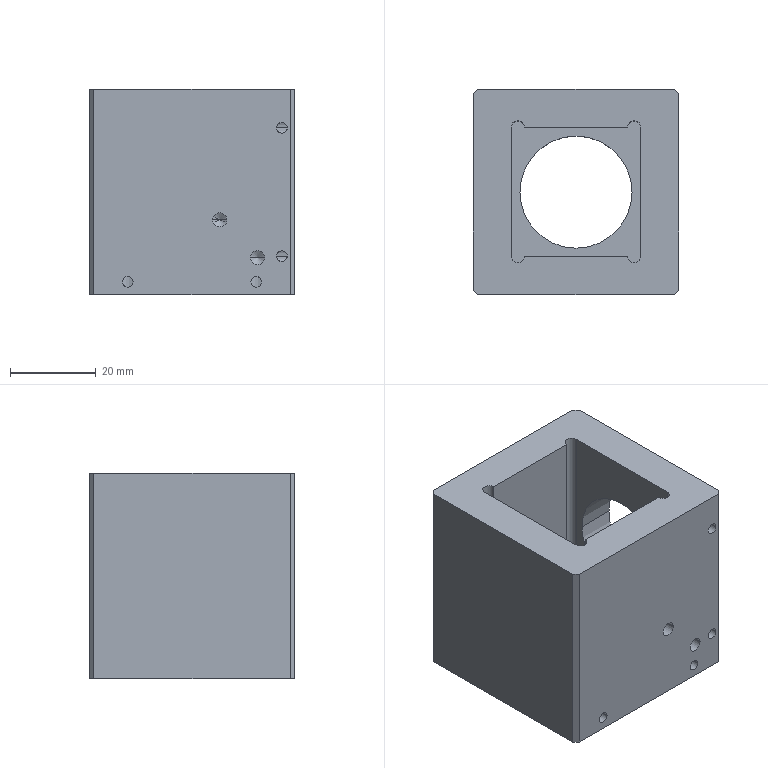Part | 1 solid | 83 faces | box 48 x 48 x 48 mm | volume 62937 mm3 | cylinder 50 | plane 23 | cone 10 | commonest cylinder face diameters 2.5 x16 6 x16 3.3 x10 3 x4 26.2 x4